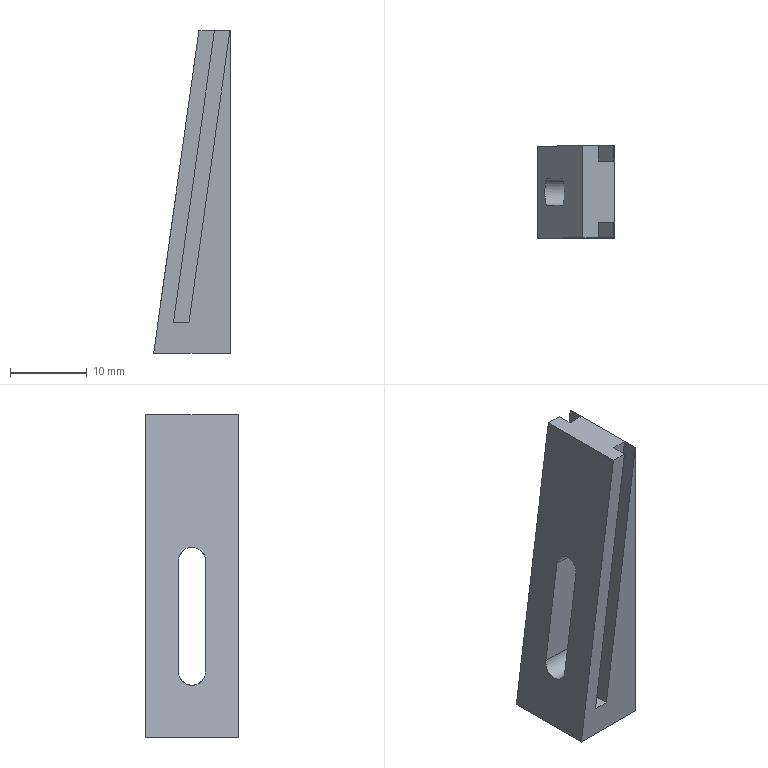Part | STEP file | SLIDE2LIFTER2_id602_x_t | 1 solid | 23 faces | box 10 x 12 x 42 mm | volume 2766 mm3 | plane 17 | cylinder 4 | other 2 | commonest cylinder face diameters 3.5 x2 2.036 x1 3.359 x1
STEP:
#1=CARTESIAN_POINT('',(18.559,1.68,18.567));
#2=VERTEX_POINT('',#1);
#3=CARTESIAN_POINT('',(18.559,1.68,18.143));
#4=VERTEX_POINT('',#3);
#5=CARTESIAN_POINT('',(18.559,1.68,14.448));
#6=DIRECTION('',(0.,0.,-1.));
#7=VECTOR('',#6,1.);
#8=LINE('',#5,#7);
#9=EDGE_CURVE('',#2,#4,#8,.T.);
#10=ORIENTED_EDGE('',*,*,#9,.F.);
#11=CARTESIAN_POINT('',(18.559,-1.68,18.567));
#12=VERTEX_POINT('',#11);
#13=CARTESIAN_POINT('',(18.559,0.,18.567));
#14=DIRECTION('',(0.,0.,1.));
#15=DIRECTION('',(0.9899,-0.1419,0.));
#16=AXIS2_PLACEMENT_3D('',#13,#14,#15);
#17=CIRCLE('',#16,1.68);
#18=EDGE_CURVE('',#2,#12,#17,.T.);
#19=ORIENTED_EDGE('',*,*,#18,.T.);
#20=CARTESIAN_POINT('',(18.559,-1.68,18.143));
#21=VERTEX_POINT('',#20);
#22=CARTESIAN_POINT('',(18.559,-1.68,14.448));
#23=DIRECTION('',(0.,0.,1.));
#24=VECTOR('',#23,1.);
#25=LINE('',#22,#24);
#26=EDGE_CURVE('',#21,#12,#25,.T.);
#27=ORIENTED_EDGE('',*,*,#26,.F.);
#28=CARTESIAN_POINT('',(18.559,0.,18.143));
#29=DIRECTION('',(0.,0.,-1.));
#30=DIRECTION('',(1.,0.,0.));
#31=AXIS2_PLACEMENT_3D('',#28,#29,#30);
#32=CIRCLE('',#31,1.68);
#33=EDGE_CURVE('',#21,#4,#32,.T.);
#34=ORIENTED_EDGE('',*,*,#33,.T.);
#35=EDGE_LOOP('',(#10,#19,#27,#34));
#36=FACE_OUTER_BOUND('',#35,.T.);
#37=CARTESIAN_POINT('',(18.559,0.,14.448));
#38=DIRECTION('',(0.,0.,1.));
#39=DIRECTION('',(1.,0.,0.));
#40=AXIS2_PLACEMENT_3D('',#37,#38,#39);
#41=CYLINDRICAL_SURFACE('',#40,1.68);
#42=ADVANCED_FACE('',(#36),#41,.F.);
#43=CARTESIAN_POINT('',(18.559,1.407,19.018));
#44=VERTEX_POINT('',#43);
#45=CARTESIAN_POINT('',(18.559,-1.407,19.018));
#46=VERTEX_POINT('',#45);
#47=CARTESIAN_POINT('',(18.559,0.,19.018));
#48=DIRECTION('',(0.,0.,1.));
#49=DIRECTION('',(0.9899,-0.1419,0.));
#50=AXIS2_PLACEMENT_3D('',#47,#48,#49);
#51=CIRCLE('',#50,1.407);
#52=EDGE_CURVE('',#44,#46,#51,.T.);
#53=ORIENTED_EDGE('',*,*,#52,.T.);
#54=CARTESIAN_POINT('',(18.559,-1.68,18.567));
#55=CARTESIAN_POINT('',(18.559,-1.68,18.624));
#56=CARTESIAN_POINT('',(18.559,-1.67,18.682));
#57=CARTESIAN_POINT('',(18.559,-1.651,18.736));
#58=CARTESIAN_POINT('',(18.559,-1.632,18.789));
#59=CARTESIAN_POINT('',(18.559,-1.604,18.841));
#60=CARTESIAN_POINT('',(18.559,-1.568,18.885));
#61=CARTESIAN_POINT('',(18.559,-1.533,18.93));
#62=CARTESIAN_POINT('',(18.559,-1.489,18.969));
#63=CARTESIAN_POINT('',(18.559,-1.441,18.999));
#64=CARTESIAN_POINT('',(18.559,-1.43,19.006));
#65=CARTESIAN_POINT('',(18.559,-1.419,19.012));
#66=CARTESIAN_POINT('',(18.559,-1.407,19.018));
#67=B_SPLINE_CURVE_WITH_KNOTS('',3,(#54,#55,#56,#57,#58,#59,#60,#61,#62,#63,#64,#65,#66),.UNSPECIFIED.,.F.,.F.,(4,3,3,3,4),(0.,0.3105,0.6211,0.9316,1.),.UNSPECIFIED.);
#68=EDGE_CURVE('',#12,#46,#67,.T.);
#69=ORIENTED_EDGE('',*,*,#68,.F.);
#70=ORIENTED_EDGE('',*,*,#18,.F.);
#71=CARTESIAN_POINT('',(18.559,1.407,19.018));
#72=CARTESIAN_POINT('',(18.559,1.458,18.991));
#73=CARTESIAN_POINT('',(18.559,1.504,18.956));
#74=CARTESIAN_POINT('',(18.559,1.543,18.914));
#75=CARTESIAN_POINT('',(18.559,1.582,18.872));
#76=CARTESIAN_POINT('',(18.559,1.614,18.823));
#77=CARTESIAN_POINT('',(18.559,1.637,18.771));
#78=CARTESIAN_POINT('',(18.559,1.66,18.719));
#79=CARTESIAN_POINT('',(18.559,1.674,18.662));
#80=CARTESIAN_POINT('',(18.559,1.678,18.605));
#81=CARTESIAN_POINT('',(18.559,1.679,18.593));
#82=CARTESIAN_POINT('',(18.559,1.68,18.58));
#83=CARTESIAN_POINT('',(18.559,1.68,18.567));
#84=B_SPLINE_CURVE_WITH_KNOTS('',3,(#71,#72,#73,#74,#75,#76,#77,#78,#79,#80,#81,#82,#83),.UNSPECIFIED.,.F.,.F.,(4,3,3,3,4),(0.,0.3105,0.6211,0.9317,1.),.UNSPECIFIED.);
#85=EDGE_CURVE('',#44,#2,#84,.T.);
#86=ORIENTED_EDGE('',*,*,#85,.F.);
#87=EDGE_LOOP('',(#53,#69,#70,#86));
#88=FACE_OUTER_BOUND('',#87,.T.);
#89=CARTESIAN_POINT('',(19.717,-0.1661,18.567));
#90=DIRECTION('',(-0.1419,-0.9899,0.));
#91=DIRECTION('',(0.9899,-0.1419,0.));
#92=AXIS2_PLACEMENT_3D('',#89,#90,#91);
#93=CIRCLE('',#92,0.509);
#94=CARTESIAN_POINT('',(18.559,0.,18.567));
#95=DIRECTION('',(0.,0.,-1.));
#96=AXIS1_PLACEMENT('',#94,#95);
#97=SURFACE_OF_REVOLUTION('',#93,#96);
#98=ADVANCED_FACE('',(#88),#97,.T.);
#99=CARTESIAN_POINT('',(18.559,-1.018,18.143));
#100=VERTEX_POINT('',#99);
#101=CARTESIAN_POINT('',(18.559,0.,18.143));
#102=DIRECTION('',(0.,-1.,0.));
#103=VECTOR('',#102,1.);
#104=LINE('',#101,#103);
#105=EDGE_CURVE('',#100,#21,#104,.T.);
#106=ORIENTED_EDGE('',*,*,#105,.F.);
#107=CARTESIAN_POINT('',(18.559,1.018,18.143));
#108=VERTEX_POINT('',#107);
#109=CARTESIAN_POINT('',(18.559,0.,18.143));
#110=DIRECTION('',(0.,0.,-1.));
#111=DIRECTION('',(-1.,0.,0.));
#112=AXIS2_PLACEMENT_3D('',#109,#110,#111);
#113=CIRCLE('',#112,1.018);
#114=EDGE_CURVE('',#100,#108,#113,.T.);
#115=ORIENTED_EDGE('',*,*,#114,.T.);
#116=CARTESIAN_POINT('',(18.559,0.,18.143));
#117=DIRECTION('',(0.,-1.,0.));
#118=VECTOR('',#117,1.);
#119=LINE('',#116,#118);
#120=EDGE_CURVE('',#4,#108,#119,.T.);
#121=ORIENTED_EDGE('',*,*,#120,.F.);
#122=ORIENTED_EDGE('',*,*,#33,.F.);
#123=EDGE_LOOP('',(#106,#115,#121,#122));
#124=FACE_OUTER_BOUND('',#123,.T.);
#125=CARTESIAN_POINT('',(18.559,0.,18.143));
#126=DIRECTION('',(0.,0.,-1.));
#127=DIRECTION('',(-1.,0.,0.));
#128=AXIS2_PLACEMENT_3D('',#125,#126,#127);
#129=PLANE('',#128);
#130=ADVANCED_FACE('',(#124),#129,.F.);
#131=ORIENTED_EDGE('',*,*,#52,.F.);
#132=CARTESIAN_POINT('',(18.559,1.407,19.018));
#133=CARTESIAN_POINT('',(18.559,1.108,19.175));
#134=CARTESIAN_POINT('',(18.559,0.7765,19.283));
#135=CARTESIAN_POINT('',(18.559,0.4414,19.333));
#136=CARTESIAN_POINT('',(18.559,0.1064,19.382));
#137=CARTESIAN_POINT('',(18.559,-0.2419,19.374));
#138=CARTESIAN_POINT('',(18.559,-0.5744,19.31));
#139=CARTESIAN_POINT('',(18.559,-0.8633,19.254));
#140=CARTESIAN_POINT('',(18.559,-1.147,19.155));
#141=CARTESIAN_POINT('',(18.559,-1.407,19.018));
#142=B_SPLINE_CURVE_WITH_KNOTS('',3,(#132,#133,#134,#135,#136,#137,#138,#139,#140,#141),.UNSPECIFIED.,.F.,.F.,(4,3,3,4),(0.,0.3489,0.6979,1.),.UNSPECIFIED.);
#143=EDGE_CURVE('',#44,#46,#142,.T.);
#144=ORIENTED_EDGE('',*,*,#143,.T.);
#145=EDGE_LOOP('',(#131,#144));
#146=FACE_OUTER_BOUND('',#145,.T.);
#147=CARTESIAN_POINT('',(18.559,-1.419,19.012));
#148=CARTESIAN_POINT('',(18.559,-2.327,18.53));
#149=CARTESIAN_POINT('',(18.559,-2.902,17.678));
#150=CARTESIAN_POINT('',(18.559,-3.009,16.656));
#151=(BOUNDED_CURVE()B_SPLINE_CURVE(3,(#147,#148,#149,#150),.UNSPECIFIED.,.F.,.F.)B_SPLINE_CURVE_WITH_KNOTS((4,4),(0.,1.),.UNSPECIFIED.)CURVE()GEOMETRIC_REPRESENTATION_ITEM()RATIONAL_B_SPLINE_CURVE((1.,0.9219,0.9219,1.))REPRESENTATION_ITEM(''));
#152=CARTESIAN_POINT('',(18.559,0.,16.339));
#153=DIRECTION('',(0.,-0.4689,0.8832));
#154=AXIS1_PLACEMENT('',#152,#153);
#155=SURFACE_OF_REVOLUTION('',#151,#154);
#156=ADVANCED_FACE('',(#146),#155,.T.);
#157=CARTESIAN_POINT('',(11.14,-6.,18.682));
#158=VERTEX_POINT('',#157);
#159=CARTESIAN_POINT('',(11.14,-4.,18.682));
#160=VERTEX_POINT('',#159);
#161=CARTESIAN_POINT('',(11.14,-6.,18.682));
#162=DIRECTION('',(0.,1.,0.));
#163=VECTOR('',#162,1.);
#164=LINE('',#161,#163);
#165=EDGE_CURVE('',#158,#160,#164,.T.);
#166=ORIENTED_EDGE('',*,*,#165,.F.);
#167=CARTESIAN_POINT('',(13.16,-6.,18.682));
#168=VERTEX_POINT('',#167);
#169=CARTESIAN_POINT('',(37.117,-6.,18.682));
#170=DIRECTION('',(-1.,0.,0.));
#171=VECTOR('',#170,1.);
#172=LINE('',#169,#171);
#173=EDGE_CURVE('',#168,#158,#172,.T.);
#174=ORIENTED_EDGE('',*,*,#173,.F.);
#175=CARTESIAN_POINT('',(13.16,-4.,18.682));
#176=VERTEX_POINT('',#175);
#177=CARTESIAN_POINT('',(13.16,-6.,18.682));
#178=DIRECTION('',(0.,-1.,0.));
#179=VECTOR('',#178,1.);
#180=LINE('',#177,#179);
#181=EDGE_CURVE('',#176,#168,#180,.T.);
#182=ORIENTED_EDGE('',*,*,#181,.F.);
#183=CARTESIAN_POINT('',(8.559,-4.,18.682));
#184=DIRECTION('',(-1.,0.,0.));
#185=VECTOR('',#184,1.);
#186=LINE('',#183,#185);
#187=EDGE_CURVE('',#176,#160,#186,.T.);
#188=ORIENTED_EDGE('',*,*,#187,.T.);
#189=EDGE_LOOP('',(#166,#174,#182,#188));
#190=FACE_OUTER_BOUND('',#189,.T.);
#191=CARTESIAN_POINT('',(13.16,-6.,18.682));
#192=DIRECTION('',(0.,0.,1.));
#193=DIRECTION('',(1.,0.,0.));
#194=AXIS2_PLACEMENT_3D('',#191,#192,#193);
#195=PLANE('',#194);
#196=ADVANCED_FACE('',(#190),#195,.T.);
#197=ORIENTED_EDGE('',*,*,#114,.F.);
#198=CARTESIAN_POINT('',(18.559,-1.018,14.682));
#199=VERTEX_POINT('',#198);
#200=CARTESIAN_POINT('',(18.559,-1.018,14.682));
#201=DIRECTION('',(0.,0.,-1.));
#202=VECTOR('',#201,1.);
#203=LINE('',#200,#202);
#204=EDGE_CURVE('',#100,#199,#203,.T.);
#205=ORIENTED_EDGE('',*,*,#204,.T.);
#206=CARTESIAN_POINT('',(18.559,1.018,14.682));
#207=VERTEX_POINT('',#206);
#208=CARTESIAN_POINT('',(18.559,0.,14.682));
#209=DIRECTION('',(0.,0.,-1.));
#210=DIRECTION('',(-1.,0.,0.));
#211=AXIS2_PLACEMENT_3D('',#208,#209,#210);
#212=CIRCLE('',#211,1.018);
#213=EDGE_CURVE('',#199,#207,#212,.T.);
#214=ORIENTED_EDGE('',*,*,#213,.T.);
#215=CARTESIAN_POINT('',(18.559,1.018,14.682));
#216=DIRECTION('',(0.,0.,1.));
#217=VECTOR('',#216,1.);
#218=LINE('',#215,#217);
#219=EDGE_CURVE('',#207,#108,#218,.T.);
#220=ORIENTED_EDGE('',*,*,#219,.T.);
#221=EDGE_LOOP('',(#197,#205,#214,#220));
#222=FACE_OUTER_BOUND('',#221,.T.);
#223=CARTESIAN_POINT('',(18.559,0.,14.448));
#224=DIRECTION('',(0.,0.,-1.));
#225=DIRECTION('',(-1.,0.,0.));
#226=AXIS2_PLACEMENT_3D('',#223,#224,#225);
#227=CYLINDRICAL_SURFACE('',#226,1.018);
#228=ADVANCED_FACE('',(#222),#227,.F.);
#229=CARTESIAN_POINT('',(13.16,6.,18.682));
#230=VERTEX_POINT('',#229);
#231=CARTESIAN_POINT('',(13.16,4.,18.682));
#232=VERTEX_POINT('',#231);
#233=CARTESIAN_POINT('',(13.16,6.,18.682));
#234=DIRECTION('',(0.,-1.,0.));
#235=VECTOR('',#234,1.);
#236=LINE('',#233,#235);
#237=EDGE_CURVE('',#230,#232,#236,.T.);
#238=ORIENTED_EDGE('',*,*,#237,.F.);
#239=CARTESIAN_POINT('',(11.14,6.,18.682));
#240=VERTEX_POINT('',#239);
#241=CARTESIAN_POINT('',(37.117,6.,18.682));
#242=DIRECTION('',(-1.,0.,0.));
#243=VECTOR('',#242,1.);
#244=LINE('',#241,#243);
#245=EDGE_CURVE('',#230,#240,#244,.T.);
#246=ORIENTED_EDGE('',*,*,#245,.T.);
#247=CARTESIAN_POINT('',(11.14,4.,18.682));
#248=VERTEX_POINT('',#247);
#249=CARTESIAN_POINT('',(11.14,6.,18.682));
#250=DIRECTION('',(0.,1.,0.));
#251=VECTOR('',#250,1.);
#252=LINE('',#249,#251);
#253=EDGE_CURVE('',#248,#240,#252,.T.);
#254=ORIENTED_EDGE('',*,*,#253,.F.);
#255=CARTESIAN_POINT('',(8.559,4.,18.682));
#256=DIRECTION('',(1.,0.,0.));
#257=VECTOR('',#256,1.);
#258=LINE('',#255,#257);
#259=EDGE_CURVE('',#248,#232,#258,.T.);
#260=ORIENTED_EDGE('',*,*,#259,.T.);
#261=EDGE_LOOP('',(#238,#246,#254,#260));
#262=FACE_OUTER_BOUND('',#261,.T.);
#263=CARTESIAN_POINT('',(11.14,6.,18.682));
#264=DIRECTION('',(0.,0.,1.));
#265=DIRECTION('',(1.,0.,0.));
#266=AXIS2_PLACEMENT_3D('',#263,#264,#265);
#267=PLANE('',#266);
#268=ADVANCED_FACE('',(#262),#267,.T.);
#269=ORIENTED_EDGE('',*,*,#187,.F.);
#270=CARTESIAN_POINT('',(18.501,-4.,56.682));
#271=VERTEX_POINT('',#270);
#272=CARTESIAN_POINT('',(18.501,-4.,56.682));
#273=DIRECTION('',(-0.1392,0.,-0.9903));
#274=VECTOR('',#273,1.);
#275=LINE('',#272,#274);
#276=EDGE_CURVE('',#271,#176,#275,.T.);
#277=ORIENTED_EDGE('',*,*,#276,.F.);
#278=CARTESIAN_POINT('',(16.481,-4.,56.682));
#279=VERTEX_POINT('',#278);
#280=CARTESIAN_POINT('',(18.559,-4.,56.682));
#281=DIRECTION('',(-1.,0.,0.));
#282=VECTOR('',#281,1.);
#283=LINE('',#280,#282);
#284=EDGE_CURVE('',#271,#279,#283,.T.);
#285=ORIENTED_EDGE('',*,*,#284,.T.);
#286=CARTESIAN_POINT('',(11.14,-4.,18.682));
#287=DIRECTION('',(0.1392,0.,0.9903));
#288=VECTOR('',#287,1.);
#289=LINE('',#286,#288);
#290=EDGE_CURVE('',#160,#279,#289,.T.);
#291=ORIENTED_EDGE('',*,*,#290,.F.);
#292=EDGE_LOOP('',(#269,#277,#285,#291));
#293=FACE_OUTER_BOUND('',#292,.T.);
#294=CARTESIAN_POINT('',(8.559,-4.,14.682));
#295=DIRECTION('',(0.,1.,0.));
#296=DIRECTION('',(0.,0.,1.));
#297=AXIS2_PLACEMENT_3D('',#294,#295,#296);
#298=PLANE('',#297);
#299=ADVANCED_FACE('',(#293),#298,.F.);
#300=CARTESIAN_POINT('',(16.481,-6.,56.682));
#301=VERTEX_POINT('',#300);
#302=CARTESIAN_POINT('',(16.481,-6.,56.682));
#303=DIRECTION('',(0.,-1.,0.));
#304=VECTOR('',#303,1.);
#305=LINE('',#302,#304);
#306=EDGE_CURVE('',#279,#301,#305,.T.);
#307=ORIENTED_EDGE('',*,*,#306,.T.);
#308=CARTESIAN_POINT('',(11.14,-6.,18.682));
#309=DIRECTION('',(0.1392,0.,0.9903));
#310=VECTOR('',#309,1.);
#311=LINE('',#308,#310);
#312=EDGE_CURVE('',#158,#301,#311,.T.);
#313=ORIENTED_EDGE('',*,*,#312,.F.);
#314=ORIENTED_EDGE('',*,*,#165,.T.);
#315=ORIENTED_EDGE('',*,*,#290,.T.);
#316=EDGE_LOOP('',(#307,#313,#314,#315));
#317=FACE_OUTER_BOUND('',#316,.T.);
#318=CARTESIAN_POINT('',(11.14,-6.,18.682));
#319=DIRECTION('',(0.9903,0.,-0.1392));
#320=DIRECTION('',(-0.1392,0.,-0.9903));
#321=AXIS2_PLACEMENT_3D('',#318,#319,#320);
#322=PLANE('',#321);
#323=ADVANCED_FACE('',(#317),#322,.T.);
#324=ORIENTED_EDGE('',*,*,#253,.T.);
#325=CARTESIAN_POINT('',(16.481,6.,56.682));
#326=VERTEX_POINT('',#325);
#327=CARTESIAN_POINT('',(11.14,6.,18.682));
#328=DIRECTION('',(0.1392,0.,0.9903));
#329=VECTOR('',#328,1.);
#330=LINE('',#327,#329);
#331=EDGE_CURVE('',#240,#326,#330,.T.);
#332=ORIENTED_EDGE('',*,*,#331,.T.);
#333=CARTESIAN_POINT('',(16.481,4.,56.682));
#334=VERTEX_POINT('',#333);
#335=CARTESIAN_POINT('',(16.481,-6.,56.682));
#336=DIRECTION('',(0.,-1.,0.));
#337=VECTOR('',#336,1.);
#338=LINE('',#335,#337);
#339=EDGE_CURVE('',#326,#334,#338,.T.);
#340=ORIENTED_EDGE('',*,*,#339,.T.);
#341=CARTESIAN_POINT('',(16.481,4.,56.682));
#342=DIRECTION('',(-0.1392,0.,-0.9903));
#343=VECTOR('',#342,1.);
#344=LINE('',#341,#343);
#345=EDGE_CURVE('',#334,#248,#344,.T.);
#346=ORIENTED_EDGE('',*,*,#345,.T.);
#347=EDGE_LOOP('',(#324,#332,#340,#346));
#348=FACE_OUTER_BOUND('',#347,.T.);
#349=CARTESIAN_POINT('',(16.481,6.,56.682));
#350=DIRECTION('',(0.9903,0.,-0.1392));
#351=DIRECTION('',(-0.1392,0.,-0.9903));
#352=AXIS2_PLACEMENT_3D('',#349,#350,#351);
#353=PLANE('',#352);
#354=ADVANCED_FACE('',(#348),#353,.T.);
#355=ORIENTED_EDGE('',*,*,#259,.F.);
#356=ORIENTED_EDGE('',*,*,#345,.F.);
#357=CARTESIAN_POINT('',(18.501,4.,56.682));
#358=VERTEX_POINT('',#357);
#359=CARTESIAN_POINT('',(18.559,4.,56.682));
#360=DIRECTION('',(1.,0.,0.));
#361=VECTOR('',#360,1.);
#362=LINE('',#359,#361);
#363=EDGE_CURVE('',#334,#358,#362,.T.);
#364=ORIENTED_EDGE('',*,*,#363,.T.);
#365=CARTESIAN_POINT('',(13.16,4.,18.682));
#366=DIRECTION('',(0.1392,0.,0.9903));
#367=VECTOR('',#366,1.);
#368=LINE('',#365,#367);
#369=EDGE_CURVE('',#232,#358,#368,.T.);
#370=ORIENTED_EDGE('',*,*,#369,.F.);
#371=EDGE_LOOP('',(#355,#356,#364,#370));
#372=FACE_OUTER_BOUND('',#371,.T.);
#373=CARTESIAN_POINT('',(8.559,4.,14.682));
#374=DIRECTION('',(0.,-1.,0.));
#375=DIRECTION('',(0.,0.,-1.));
#376=AXIS2_PLACEMENT_3D('',#373,#374,#375);
#377=PLANE('',#376);
#378=ADVANCED_FACE('',(#372),#377,.F.);
#379=CARTESIAN_POINT('',(18.501,6.,56.682));
#380=VERTEX_POINT('',#379);
#381=CARTESIAN_POINT('',(18.501,-6.,56.682));
#382=DIRECTION('',(0.,1.,0.));
#383=VECTOR('',#382,1.);
#384=LINE('',#381,#383);
#385=EDGE_CURVE('',#358,#380,#384,.T.);
#386=ORIENTED_EDGE('',*,*,#385,.T.);
#387=CARTESIAN_POINT('',(18.501,6.,56.682));
#388=DIRECTION('',(-0.1392,0.,-0.9903));
#389=VECTOR('',#388,1.);
#390=LINE('',#387,#389);
#391=EDGE_CURVE('',#380,#230,#390,.T.);
#392=ORIENTED_EDGE('',*,*,#391,.T.);
#393=ORIENTED_EDGE('',*,*,#237,.T.);
#394=ORIENTED_EDGE('',*,*,#369,.T.);
#395=EDGE_LOOP('',(#386,#392,#393,#394));
#396=FACE_OUTER_BOUND('',#395,.T.);
#397=CARTESIAN_POINT('',(13.16,6.,18.682));
#398=DIRECTION('',(-0.9903,0.,0.1392));
#399=DIRECTION('',(0.1392,0.,0.9903));
#400=AXIS2_PLACEMENT_3D('',#397,#398,#399);
#401=PLANE('',#400);
#402=ADVANCED_FACE('',(#396),#401,.T.);
#403=ORIENTED_EDGE('',*,*,#181,.T.);
#404=CARTESIAN_POINT('',(18.501,-6.,56.682));
#405=VERTEX_POINT('',#404);
#406=CARTESIAN_POINT('',(18.501,-6.,56.682));
#407=DIRECTION('',(-0.1392,0.,-0.9903));
#408=VECTOR('',#407,1.);
#409=LINE('',#406,#408);
#410=EDGE_CURVE('',#405,#168,#409,.T.);
#411=ORIENTED_EDGE('',*,*,#410,.F.);
#412=CARTESIAN_POINT('',(18.501,-6.,56.682));
#413=DIRECTION('',(0.,1.,0.));
#414=VECTOR('',#413,1.);
#415=LINE('',#412,#414);
#416=EDGE_CURVE('',#405,#271,#415,.T.);
#417=ORIENTED_EDGE('',*,*,#416,.T.);
#418=ORIENTED_EDGE('',*,*,#276,.T.);
#419=EDGE_LOOP('',(#403,#411,#417,#418));
#420=FACE_OUTER_BOUND('',#419,.T.);
#421=CARTESIAN_POINT('',(18.501,-6.,56.682));
#422=DIRECTION('',(-0.9903,0.,0.1392));
#423=DIRECTION('',(0.1392,0.,0.9903));
#424=AXIS2_PLACEMENT_3D('',#421,#422,#423);
#425=PLANE('',#424);
#426=ADVANCED_FACE('',(#420),#425,.T.);
#427=CARTESIAN_POINT('',(18.559,1.75,23.182));
#428=VERTEX_POINT('',#427);
#429=CARTESIAN_POINT('',(18.559,1.75,37.682));
#430=VERTEX_POINT('',#429);
#431=CARTESIAN_POINT('',(18.559,1.75,37.682));
#432=DIRECTION('',(0.,0.,1.));
#433=VECTOR('',#432,1.);
#434=LINE('',#431,#433);
#435=EDGE_CURVE('',#428,#430,#434,.T.);
#436=ORIENTED_EDGE('',*,*,#435,.F.);
#437=CARTESIAN_POINT('',(18.559,-1.75,23.182));
#438=VERTEX_POINT('',#437);
#439=CARTESIAN_POINT('',(18.559,0.,23.182));
#440=DIRECTION('',(-1.,0.,0.));
#441=DIRECTION('',(0.,0.,1.));
#442=AXIS2_PLACEMENT_3D('',#439,#440,#441);
#443=CIRCLE('',#442,1.75);
#444=EDGE_CURVE('',#428,#438,#443,.T.);
#445=ORIENTED_EDGE('',*,*,#444,.T.);
#446=CARTESIAN_POINT('',(18.559,-1.75,37.682));
#447=VERTEX_POINT('',#446);
#448=CARTESIAN_POINT('',(18.559,-1.75,23.182));
#449=DIRECTION('',(0.,0.,-1.));
#450=VECTOR('',#449,1.);
#451=LINE('',#448,#450);
#452=EDGE_CURVE('',#447,#438,#451,.T.);
#453=ORIENTED_EDGE('',*,*,#452,.F.);
#454=CARTESIAN_POINT('',(18.559,0.,37.682));
#455=DIRECTION('',(-1.,0.,0.));
#456=DIRECTION('',(0.,0.,1.));
#457=AXIS2_PLACEMENT_3D('',#454,#455,#456);
#458=CIRCLE('',#457,1.75);
#459=EDGE_CURVE('',#447,#430,#458,.T.);
#460=ORIENTED_EDGE('',*,*,#459,.T.);
#461=EDGE_LOOP('',(#436,#445,#453,#460));
#462=FACE_BOUND('',#461,.T.);
#463=CARTESIAN_POINT('',(18.559,6.,14.682));
#464=VERTEX_POINT('',#463);
#465=CARTESIAN_POINT('',(18.559,6.,56.682));
#466=VERTEX_POINT('',#465);
#467=CARTESIAN_POINT('',(18.559,6.,0.));
#468=DIRECTION('',(0.,0.,1.));
#469=VECTOR('',#468,1.);
#470=LINE('',#467,#469);
#471=EDGE_CURVE('',#464,#466,#470,.T.);
#472=ORIENTED_EDGE('',*,*,#471,.T.);
#473=CARTESIAN_POINT('',(18.559,-6.,56.682));
#474=VERTEX_POINT('',#473);
#475=CARTESIAN_POINT('',(18.559,-6.,56.682));
#476=DIRECTION('',(0.,-1.,0.));
#477=VECTOR('',#476,1.);
#478=LINE('',#475,#477);
#479=EDGE_CURVE('',#466,#474,#478,.T.);
#480=ORIENTED_EDGE('',*,*,#479,.T.);
#481=CARTESIAN_POINT('',(18.559,-6.,14.682));
#482=VERTEX_POINT('',#481);
#483=CARTESIAN_POINT('',(18.559,-6.,0.));
#484=DIRECTION('',(0.,0.,1.));
#485=VECTOR('',#484,1.);
#486=LINE('',#483,#485);
#487=EDGE_CURVE('',#482,#474,#486,.T.);
#488=ORIENTED_EDGE('',*,*,#487,.F.);
#489=CARTESIAN_POINT('',(18.559,-6.,14.682));
#490=DIRECTION('',(0.,1.,0.));
#491=VECTOR('',#490,1.);
#492=LINE('',#489,#491);
#493=EDGE_CURVE('',#482,#199,#492,.T.);
#494=ORIENTED_EDGE('',*,*,#493,.T.);
#495=ORIENTED_EDGE('',*,*,#204,.F.);
#496=ORIENTED_EDGE('',*,*,#105,.T.);
#497=ORIENTED_EDGE('',*,*,#26,.T.);
#498=ORIENTED_EDGE('',*,*,#68,.T.);
#499=ORIENTED_EDGE('',*,*,#143,.F.);
#500=ORIENTED_EDGE('',*,*,#85,.T.);
#501=ORIENTED_EDGE('',*,*,#9,.T.);
#502=ORIENTED_EDGE('',*,*,#120,.T.);
#503=ORIENTED_EDGE('',*,*,#219,.F.);
#504=CARTESIAN_POINT('',(18.559,-6.,14.682));
#505=DIRECTION('',(0.,1.,0.));
#506=VECTOR('',#505,1.);
#507=LINE('',#504,#506);
#508=EDGE_CURVE('',#207,#464,#507,.T.);
#509=ORIENTED_EDGE('',*,*,#508,.T.);
#510=EDGE_LOOP('',(#472,#480,#488,#494,#495,#496,#497,#498,#499,#500,#501,#502,#503,#509));
#511=FACE_BOUND('',#510,.T.);
#512=CARTESIAN_POINT('',(18.559,-6.,14.682));
#513=DIRECTION('',(-1.,0.,0.));
#514=DIRECTION('',(0.,0.,1.));
#515=AXIS2_PLACEMENT_3D('',#512,#513,#514);
#516=PLANE('',#515);
#517=ADVANCED_FACE('',(#462,#511),#516,.F.);
#518=ORIENTED_EDGE('',*,*,#173,.T.);
#519=ORIENTED_EDGE('',*,*,#312,.T.);
#520=CARTESIAN_POINT('',(14.461,-6.,56.682));
#521=VERTEX_POINT('',#520);
#522=CARTESIAN_POINT('',(18.559,-6.,56.682));
#523=DIRECTION('',(-1.,0.,0.));
#524=VECTOR('',#523,1.);
#525=LINE('',#522,#524);
#526=EDGE_CURVE('',#301,#521,#525,.T.);
#527=ORIENTED_EDGE('',*,*,#526,.T.);
#528=CARTESIAN_POINT('',(8.559,-6.,14.682));
#529=VERTEX_POINT('',#528);
#530=CARTESIAN_POINT('',(14.461,-6.,56.682));
#531=DIRECTION('',(-0.1392,0.,-0.9903));
#532=VECTOR('',#531,1.);
#533=LINE('',#530,#532);
#534=EDGE_CURVE('',#521,#529,#533,.T.);
#535=ORIENTED_EDGE('',*,*,#534,.T.);
#536=CARTESIAN_POINT('',(8.559,-6.,14.682));
#537=DIRECTION('',(1.,0.,0.));
#538=VECTOR('',#537,1.);
#539=LINE('',#536,#538);
#540=EDGE_CURVE('',#529,#482,#539,.T.);
#541=ORIENTED_EDGE('',*,*,#540,.T.);
#542=ORIENTED_EDGE('',*,*,#487,.T.);
#543=CARTESIAN_POINT('',(18.559,-6.,56.682));
#544=DIRECTION('',(-1.,0.,0.));
#545=VECTOR('',#544,1.);
#546=LINE('',#543,#545);
#547=EDGE_CURVE('',#474,#405,#546,.T.);
#548=ORIENTED_EDGE('',*,*,#547,.T.);
#549=ORIENTED_EDGE('',*,*,#410,.T.);
#550=EDGE_LOOP('',(#518,#519,#527,#535,#541,#542,#548,#549));
#551=FACE_OUTER_BOUND('',#550,.T.);
#552=CARTESIAN_POINT('',(37.117,-6.,0.));
#553=DIRECTION('',(0.,-1.,0.));
#554=DIRECTION('',(0.,0.,-1.));
#555=AXIS2_PLACEMENT_3D('',#552,#553,#554);
#556=PLANE('',#555);
#557=ADVANCED_FACE('',(#551),#556,.T.);
#558=ORIENTED_EDGE('',*,*,#540,.F.);
#559=CARTESIAN_POINT('',(8.559,6.,14.682));
#560=VERTEX_POINT('',#559);
#561=CARTESIAN_POINT('',(8.559,-6.,14.682));
#562=DIRECTION('',(0.,1.,0.));
#563=VECTOR('',#562,1.);
#564=LINE('',#561,#563);
#565=EDGE_CURVE('',#529,#560,#564,.T.);
#566=ORIENTED_EDGE('',*,*,#565,.T.);
#567=CARTESIAN_POINT('',(37.117,6.,14.682));
#568=DIRECTION('',(1.,0.,0.));
#569=VECTOR('',#568,1.);
#570=LINE('',#567,#569);
#571=EDGE_CURVE('',#560,#464,#570,.T.);
#572=ORIENTED_EDGE('',*,*,#571,.T.);
#573=ORIENTED_EDGE('',*,*,#508,.F.);
#574=ORIENTED_EDGE('',*,*,#213,.F.);
#575=ORIENTED_EDGE('',*,*,#493,.F.);
#576=EDGE_LOOP('',(#558,#566,#572,#573,#574,#575));
#577=FACE_OUTER_BOUND('',#576,.T.);
#578=CARTESIAN_POINT('',(8.559,-6.,14.682));
#579=DIRECTION('',(0.,0.,1.));
#580=DIRECTION('',(1.,0.,0.));
#581=AXIS2_PLACEMENT_3D('',#578,#579,#580);
#582=PLANE('',#581);
#583=ADVANCED_FACE('',(#577),#582,.F.);
#584=ORIENTED_EDGE('',*,*,#391,.F.);
#585=CARTESIAN_POINT('',(18.559,6.,56.682));
#586=DIRECTION('',(1.,0.,0.));
#587=VECTOR('',#586,1.);
#588=LINE('',#585,#587);
#589=EDGE_CURVE('',#380,#466,#588,.T.);
#590=ORIENTED_EDGE('',*,*,#589,.T.);
#591=ORIENTED_EDGE('',*,*,#471,.F.);
#592=ORIENTED_EDGE('',*,*,#571,.F.);
#593=CARTESIAN_POINT('',(14.461,6.,56.682));
#594=VERTEX_POINT('',#593);
#595=CARTESIAN_POINT('',(14.461,6.,56.682));
#596=DIRECTION('',(0.1392,0.,0.9903));
#597=VECTOR('',#596,1.);
#598=LINE('',#595,#597);
#599=EDGE_CURVE('',#560,#594,#598,.T.);
#600=ORIENTED_EDGE('',*,*,#599,.T.);
#601=CARTESIAN_POINT('',(18.559,6.,56.682));
#602=DIRECTION('',(1.,0.,0.));
#603=VECTOR('',#602,1.);
#604=LINE('',#601,#603);
#605=EDGE_CURVE('',#594,#326,#604,.T.);
#606=ORIENTED_EDGE('',*,*,#605,.T.);
#607=ORIENTED_EDGE('',*,*,#331,.F.);
#608=ORIENTED_EDGE('',*,*,#245,.F.);
#609=EDGE_LOOP('',(#584,#590,#591,#592,#600,#606,#607,#608));
#610=FACE_OUTER_BOUND('',#609,.T.);
#611=CARTESIAN_POINT('',(37.117,6.,0.));
#612=DIRECTION('',(0.,-1.,0.));
#613=DIRECTION('',(0.,0.,-1.));
#614=AXIS2_PLACEMENT_3D('',#611,#612,#613);
#615=PLANE('',#614);
#616=ADVANCED_FACE('',(#610),#615,.F.);
#617=ORIENTED_EDGE('',*,*,#547,.F.);
#618=ORIENTED_EDGE('',*,*,#479,.F.);
#619=ORIENTED_EDGE('',*,*,#589,.F.);
#620=ORIENTED_EDGE('',*,*,#385,.F.);
#621=ORIENTED_EDGE('',*,*,#363,.F.);
#622=ORIENTED_EDGE('',*,*,#339,.F.);
#623=ORIENTED_EDGE('',*,*,#605,.F.);
#624=CARTESIAN_POINT('',(14.461,-6.,56.682));
#625=DIRECTION('',(0.,-1.,0.));
#626=VECTOR('',#625,1.);
#627=LINE('',#624,#626);
#628=EDGE_CURVE('',#594,#521,#627,.T.);
#629=ORIENTED_EDGE('',*,*,#628,.T.);
#630=ORIENTED_EDGE('',*,*,#526,.F.);
#631=ORIENTED_EDGE('',*,*,#306,.F.);
#632=ORIENTED_EDGE('',*,*,#284,.F.);
#633=ORIENTED_EDGE('',*,*,#416,.F.);
#634=EDGE_LOOP('',(#617,#618,#619,#620,#621,#622,#623,#629,#630,#631,#632,#633));
#635=FACE_OUTER_BOUND('',#634,.T.);
#636=CARTESIAN_POINT('',(18.559,-6.,56.682));
#637=DIRECTION('',(0.,0.,-1.));
#638=DIRECTION('',(-1.,0.,0.));
#639=AXIS2_PLACEMENT_3D('',#636,#637,#638);
#640=PLANE('',#639);
#641=ADVANCED_FACE('',(#635),#640,.F.);
#642=CARTESIAN_POINT('',(11.791,-1.75,37.682));
#643=VERTEX_POINT('',#642);
#644=CARTESIAN_POINT('',(18.559,-1.75,37.682));
#645=DIRECTION('',(1.,0.,0.));
#646=VECTOR('',#645,1.);
#647=LINE('',#644,#646);
#648=EDGE_CURVE('',#643,#447,#647,.T.);
#649=ORIENTED_EDGE('',*,*,#648,.T.);
#650=ORIENTED_EDGE('',*,*,#452,.T.);
#651=CARTESIAN_POINT('',(9.753,-1.75,23.182));
#652=VERTEX_POINT('',#651);
#653=CARTESIAN_POINT('',(18.559,-1.75,23.182));
#654=DIRECTION('',(-1.,0.,0.));
#655=VECTOR('',#654,1.);
#656=LINE('',#653,#655);
#657=EDGE_CURVE('',#438,#652,#656,.T.);
#658=ORIENTED_EDGE('',*,*,#657,.T.);
#659=CARTESIAN_POINT('',(14.461,-1.75,56.682));
#660=DIRECTION('',(0.1392,0.,0.9903));
#661=VECTOR('',#660,1.);
#662=LINE('',#659,#661);
#663=EDGE_CURVE('',#652,#643,#662,.T.);
#664=ORIENTED_EDGE('',*,*,#663,.T.);
#665=EDGE_LOOP('',(#649,#650,#658,#664));
#666=FACE_OUTER_BOUND('',#665,.T.);
#667=CARTESIAN_POINT('',(18.559,-1.75,23.182));
#668=DIRECTION('',(0.,1.,0.));
#669=DIRECTION('',(0.,0.,1.));
#670=AXIS2_PLACEMENT_3D('',#667,#668,#669);
#671=PLANE('',#670);
#672=ADVANCED_FACE('',(#666),#671,.T.);
#673=CARTESIAN_POINT('',(11.791,1.75,37.682));
#674=VERTEX_POINT('',#673);
#675=CARTESIAN_POINT('',(11.791,0.,37.682));
#676=DIRECTION('',(-0.9903,0.,0.1392));
#677=DIRECTION('',(-0.1392,0.,-0.9903));
#678=AXIS2_PLACEMENT_3D('',#675,#676,#677);
#679=ELLIPSE('',#678,1.767,1.75);
#680=EDGE_CURVE('',#643,#674,#679,.T.);
#681=ORIENTED_EDGE('',*,*,#680,.T.);
#682=CARTESIAN_POINT('',(18.559,1.75,37.682));
#683=DIRECTION('',(-1.,0.,0.));
#684=VECTOR('',#683,1.);
#685=LINE('',#682,#684);
#686=EDGE_CURVE('',#430,#674,#685,.T.);
#687=ORIENTED_EDGE('',*,*,#686,.F.);
#688=ORIENTED_EDGE('',*,*,#459,.F.);
#689=ORIENTED_EDGE('',*,*,#648,.F.);
#690=EDGE_LOOP('',(#681,#687,#688,#689));
#691=FACE_OUTER_BOUND('',#690,.T.);
#692=CARTESIAN_POINT('',(18.559,0.,37.682));
#693=DIRECTION('',(-1.,0.,0.));
#694=DIRECTION('',(0.,0.,1.));
#695=AXIS2_PLACEMENT_3D('',#692,#693,#694);
#696=CYLINDRICAL_SURFACE('',#695,1.75);
#697=ADVANCED_FACE('',(#691),#696,.F.);
#698=CARTESIAN_POINT('',(9.753,1.75,23.182));
#699=VERTEX_POINT('',#698);
#700=CARTESIAN_POINT('',(18.559,1.75,23.182));
#701=DIRECTION('',(1.,0.,0.));
#702=VECTOR('',#701,1.);
#703=LINE('',#700,#702);
#704=EDGE_CURVE('',#699,#428,#703,.T.);
#705=ORIENTED_EDGE('',*,*,#704,.T.);
#706=ORIENTED_EDGE('',*,*,#435,.T.);
#707=ORIENTED_EDGE('',*,*,#686,.T.);
#708=CARTESIAN_POINT('',(14.461,1.75,56.682));
#709=DIRECTION('',(-0.1392,0.,-0.9903));
#710=VECTOR('',#709,1.);
#711=LINE('',#708,#710);
#712=EDGE_CURVE('',#674,#699,#711,.T.);
#713=ORIENTED_EDGE('',*,*,#712,.T.);
#714=EDGE_LOOP('',(#705,#706,#707,#713));
#715=FACE_OUTER_BOUND('',#714,.T.);
#716=CARTESIAN_POINT('',(18.559,1.75,37.682));
#717=DIRECTION('',(0.,-1.,0.));
#718=DIRECTION('',(0.,0.,-1.));
#719=AXIS2_PLACEMENT_3D('',#716,#717,#718);
#720=PLANE('',#719);
#721=ADVANCED_FACE('',(#715),#720,.T.);
#722=CARTESIAN_POINT('',(9.753,0.,23.182));
#723=DIRECTION('',(-0.9903,0.,0.1392));
#724=DIRECTION('',(-0.1392,0.,-0.9903));
#725=AXIS2_PLACEMENT_3D('',#722,#723,#724);
#726=ELLIPSE('',#725,1.767,1.75);
#727=EDGE_CURVE('',#699,#652,#726,.T.);
#728=ORIENTED_EDGE('',*,*,#727,.T.);
#729=ORIENTED_EDGE('',*,*,#657,.F.);
#730=ORIENTED_EDGE('',*,*,#444,.F.);
#731=ORIENTED_EDGE('',*,*,#704,.F.);
#732=EDGE_LOOP('',(#728,#729,#730,#731));
#733=FACE_OUTER_BOUND('',#732,.T.);
#734=CARTESIAN_POINT('',(18.559,0.,23.182));
#735=DIRECTION('',(-1.,0.,0.));
#736=DIRECTION('',(0.,0.,1.));
#737=AXIS2_PLACEMENT_3D('',#734,#735,#736);
#738=CYLINDRICAL_SURFACE('',#737,1.75);
#739=ADVANCED_FACE('',(#733),#738,.F.);
#740=ORIENTED_EDGE('',*,*,#712,.F.);
#741=ORIENTED_EDGE('',*,*,#680,.F.);
#742=ORIENTED_EDGE('',*,*,#663,.F.);
#743=ORIENTED_EDGE('',*,*,#727,.F.);
#744=EDGE_LOOP('',(#740,#741,#742,#743));
#745=FACE_BOUND('',#744,.T.);
#746=ORIENTED_EDGE('',*,*,#599,.F.);
#747=ORIENTED_EDGE('',*,*,#565,.F.);
#748=ORIENTED_EDGE('',*,*,#534,.F.);
#749=ORIENTED_EDGE('',*,*,#628,.F.);
#750=EDGE_LOOP('',(#746,#747,#748,#749));
#751=FACE_BOUND('',#750,.T.);
#752=CARTESIAN_POINT('',(14.461,-6.,56.682));
#753=DIRECTION('',(0.9903,0.,-0.1392));
#754=DIRECTION('',(-0.1392,0.,-0.9903));
#755=AXIS2_PLACEMENT_3D('',#752,#753,#754);
#756=PLANE('',#755);
#757=ADVANCED_FACE('',(#745,#751),#756,.F.);
#758=CLOSED_SHELL('',(#42,#98,#130,#156,#196,#228,#268,#299,#323,#354,#378,#402,#426,#517,#557,#583,#616,#641,#672,#697,#721,#739,#757));
#759=MANIFOLD_SOLID_BREP('',#758);
#760=(LENGTH_UNIT()NAMED_UNIT(*)SI_UNIT(.MILLI.,.METRE.));
#761=UNCERTAINTY_MEASURE_WITH_UNIT(LENGTH_MEASURE(0.0508),#760,'','');
#762=(NAMED_UNIT(*)PLANE_ANGLE_UNIT()SI_UNIT($,.RADIAN.));
#763=PLANE_ANGLE_MEASURE_WITH_UNIT(PLANE_ANGLE_MEASURE(0.01745),#762);
#764=DIMENSIONAL_EXPONENTS(0.,0.,0.,0.,0.,0.,0.);
#765=(CONVERSION_BASED_UNIT('DEGREE',#763)NAMED_UNIT(#764)PLANE_ANGLE_UNIT());
#766=(NAMED_UNIT(*)SI_UNIT($,.STERADIAN.)SOLID_ANGLE_UNIT());
#767=(GEOMETRIC_REPRESENTATION_CONTEXT(3)GLOBAL_UNCERTAINTY_ASSIGNED_CONTEXT((#761))GLOBAL_UNIT_ASSIGNED_CONTEXT((#760,#765,#766))REPRESENTATION_CONTEXT('',''));
#768=ADVANCED_BREP_SHAPE_REPRESENTATION('',(#759),#767);